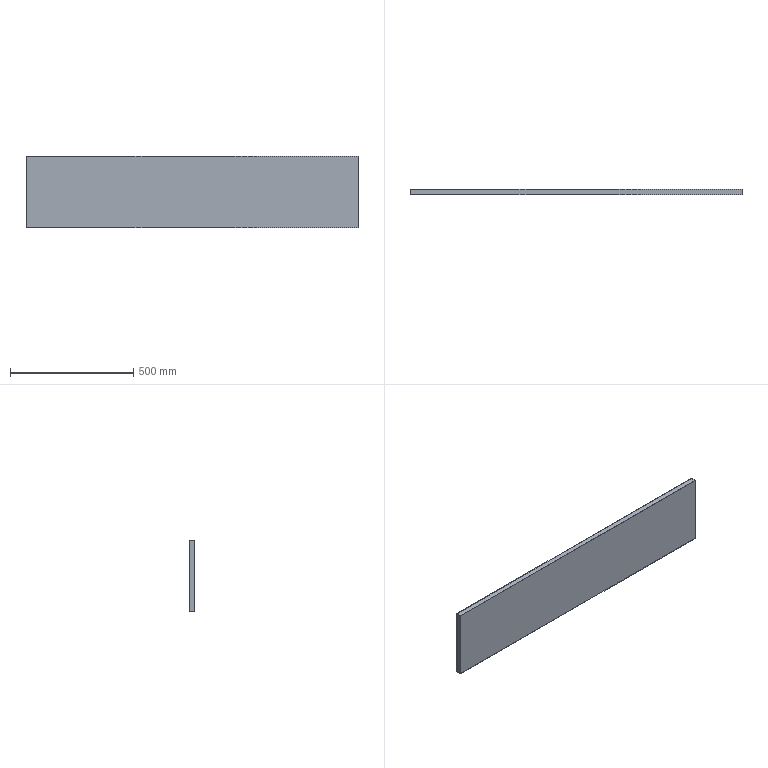Part | SolidWorks | features Extrusion 1, ICE 1, Shell 1 | 1 solid | 12 faces | box 1346 x 22 x 288 mm | volume 1667952 mm3 | plane 12
STEP:
#1=CARTESIAN_POINT('',(-673.,0.,-144.));
#2=VERTEX_POINT('',#1);
#3=CARTESIAN_POINT('',(-673.,0.,144.));
#4=VERTEX_POINT('',#3);
#5=CARTESIAN_POINT('',(-673.,0.,-144.));
#6=DIRECTION('',(0.,0.,1.));
#7=VECTOR('',#6,1000.);
#8=LINE('',#5,#7);
#9=EDGE_CURVE('',#2,#4,#8,.T.);
#10=ORIENTED_EDGE('',*,*,#9,.F.);
#11=CARTESIAN_POINT('',(-673.,-22.,-144.));
#12=VERTEX_POINT('',#11);
#13=CARTESIAN_POINT('',(-673.,-20.,-144.));
#14=DIRECTION('',(0.,1.,0.));
#15=VECTOR('',#14,1000.);
#16=LINE('',#13,#15);
#17=EDGE_CURVE('',#12,#2,#16,.T.);
#18=ORIENTED_EDGE('',*,*,#17,.F.);
#19=CARTESIAN_POINT('',(-673.,-22.,144.));
#20=VERTEX_POINT('',#19);
#21=CARTESIAN_POINT('',(-673.,-22.,144.));
#22=DIRECTION('',(0.,0.,-1.));
#23=VECTOR('',#22,1000.);
#24=LINE('',#21,#23);
#25=EDGE_CURVE('',#20,#12,#24,.T.);
#26=ORIENTED_EDGE('',*,*,#25,.F.);
#27=CARTESIAN_POINT('',(-673.,-20.,144.));
#28=DIRECTION('',(0.,1.,0.));
#29=VECTOR('',#28,1000.);
#30=LINE('',#27,#29);
#31=EDGE_CURVE('',#20,#4,#30,.T.);
#32=ORIENTED_EDGE('',*,*,#31,.T.);
#33=EDGE_LOOP('',(#10,#18,#26,#32));
#34=FACE_OUTER_BOUND('',#33,.T.);
#35=CARTESIAN_POINT('',(-673.,-20.,-144.));
#36=DIRECTION('',(-1.,0.,0.));
#37=DIRECTION('',(0.,0.,1.));
#38=AXIS2_PLACEMENT_3D('',#35,#36,#37);
#39=PLANE('',#38);
#40=ADVANCED_FACE('',(#34),#39,.T.);
#41=CARTESIAN_POINT('',(673.,0.,-144.));
#42=VERTEX_POINT('',#41);
#43=CARTESIAN_POINT('',(-673.,0.,-144.));
#44=DIRECTION('',(-1.,0.,0.));
#45=VECTOR('',#44,1000.);
#46=LINE('',#43,#45);
#47=EDGE_CURVE('',#42,#2,#46,.T.);
#48=ORIENTED_EDGE('',*,*,#47,.F.);
#49=CARTESIAN_POINT('',(673.,-22.,-144.));
#50=VERTEX_POINT('',#49);
#51=CARTESIAN_POINT('',(673.,-20.,-144.));
#52=DIRECTION('',(0.,1.,0.));
#53=VECTOR('',#52,1000.);
#54=LINE('',#51,#53);
#55=EDGE_CURVE('',#50,#42,#54,.T.);
#56=ORIENTED_EDGE('',*,*,#55,.F.);
#57=CARTESIAN_POINT('',(-673.,-22.,-144.));
#58=DIRECTION('',(1.,0.,0.));
#59=VECTOR('',#58,1000.);
#60=LINE('',#57,#59);
#61=EDGE_CURVE('',#12,#50,#60,.T.);
#62=ORIENTED_EDGE('',*,*,#61,.F.);
#63=ORIENTED_EDGE('',*,*,#17,.T.);
#64=EDGE_LOOP('',(#48,#56,#62,#63));
#65=FACE_OUTER_BOUND('',#64,.T.);
#66=CARTESIAN_POINT('',(-673.,-20.,-144.));
#67=DIRECTION('',(0.,0.,-1.));
#68=DIRECTION('',(-1.,0.,0.));
#69=AXIS2_PLACEMENT_3D('',#66,#67,#68);
#70=PLANE('',#69);
#71=ADVANCED_FACE('',(#65),#70,.T.);
#72=CARTESIAN_POINT('',(673.,0.,144.));
#73=VERTEX_POINT('',#72);
#74=CARTESIAN_POINT('',(673.,0.,-144.));
#75=DIRECTION('',(0.,0.,-1.));
#76=VECTOR('',#75,1000.);
#77=LINE('',#74,#76);
#78=EDGE_CURVE('',#73,#42,#77,.T.);
#79=ORIENTED_EDGE('',*,*,#78,.F.);
#80=CARTESIAN_POINT('',(673.,-22.,144.));
#81=VERTEX_POINT('',#80);
#82=CARTESIAN_POINT('',(673.,-20.,144.));
#83=DIRECTION('',(0.,1.,0.));
#84=VECTOR('',#83,1000.);
#85=LINE('',#82,#84);
#86=EDGE_CURVE('',#81,#73,#85,.T.);
#87=ORIENTED_EDGE('',*,*,#86,.F.);
#88=CARTESIAN_POINT('',(673.,-22.,144.));
#89=DIRECTION('',(0.,0.,1.));
#90=VECTOR('',#89,1000.);
#91=LINE('',#88,#90);
#92=EDGE_CURVE('',#50,#81,#91,.T.);
#93=ORIENTED_EDGE('',*,*,#92,.F.);
#94=ORIENTED_EDGE('',*,*,#55,.T.);
#95=EDGE_LOOP('',(#79,#87,#93,#94));
#96=FACE_OUTER_BOUND('',#95,.T.);
#97=CARTESIAN_POINT('',(673.,-20.,-144.));
#98=DIRECTION('',(1.,0.,0.));
#99=DIRECTION('',(0.,0.,-1.));
#100=AXIS2_PLACEMENT_3D('',#97,#98,#99);
#101=PLANE('',#100);
#102=ADVANCED_FACE('',(#96),#101,.T.);
#103=CARTESIAN_POINT('',(-673.,0.,144.));
#104=DIRECTION('',(1.,0.,0.));
#105=VECTOR('',#104,1000.);
#106=LINE('',#103,#105);
#107=EDGE_CURVE('',#4,#73,#106,.T.);
#108=ORIENTED_EDGE('',*,*,#107,.F.);
#109=ORIENTED_EDGE('',*,*,#31,.F.);
#110=CARTESIAN_POINT('',(-673.,-22.,144.));
#111=DIRECTION('',(-1.,0.,0.));
#112=VECTOR('',#111,1000.);
#113=LINE('',#110,#112);
#114=EDGE_CURVE('',#81,#20,#113,.T.);
#115=ORIENTED_EDGE('',*,*,#114,.F.);
#116=ORIENTED_EDGE('',*,*,#86,.T.);
#117=EDGE_LOOP('',(#108,#109,#115,#116));
#118=FACE_OUTER_BOUND('',#117,.T.);
#119=CARTESIAN_POINT('',(-673.,-20.,144.));
#120=DIRECTION('',(0.,0.,1.));
#121=DIRECTION('',(1.,0.,0.));
#122=AXIS2_PLACEMENT_3D('',#119,#120,#121);
#123=PLANE('',#122);
#124=ADVANCED_FACE('',(#118),#123,.T.);
#125=ORIENTED_EDGE('',*,*,#9,.T.);
#126=ORIENTED_EDGE('',*,*,#107,.T.);
#127=ORIENTED_EDGE('',*,*,#78,.T.);
#128=ORIENTED_EDGE('',*,*,#47,.T.);
#129=EDGE_LOOP('',(#125,#126,#127,#128));
#130=FACE_OUTER_BOUND('',#129,.T.);
#131=CARTESIAN_POINT('',(-673.,0.,144.));
#132=DIRECTION('',(0.,1.,0.));
#133=DIRECTION('',(0.,0.,1.));
#134=AXIS2_PLACEMENT_3D('',#131,#132,#133);
#135=PLANE('',#134);
#136=ADVANCED_FACE('',(#130),#135,.T.);
#137=ORIENTED_EDGE('',*,*,#25,.T.);
#138=ORIENTED_EDGE('',*,*,#61,.T.);
#139=ORIENTED_EDGE('',*,*,#92,.T.);
#140=ORIENTED_EDGE('',*,*,#114,.T.);
#141=EDGE_LOOP('',(#137,#138,#139,#140));
#142=FACE_OUTER_BOUND('',#141,.T.);
#143=CARTESIAN_POINT('',(-673.,-22.,-144.));
#144=DIRECTION('',(0.,-1.,0.));
#145=DIRECTION('',(0.,0.,-1.));
#146=AXIS2_PLACEMENT_3D('',#143,#144,#145);
#147=PLANE('',#146);
#148=ADVANCED_FACE('',(#142),#147,.T.);
#149=CLOSED_SHELL('',(#40,#71,#102,#124,#136,#148));
#150=CARTESIAN_POINT('',(671.,-20.,-142.));
#151=VERTEX_POINT('',#150);
#152=CARTESIAN_POINT('',(-671.,-20.,-142.));
#153=VERTEX_POINT('',#152);
#154=CARTESIAN_POINT('',(-673.,-20.,-142.));
#155=DIRECTION('',(-1.,0.,0.));
#156=VECTOR('',#155,1000.);
#157=LINE('',#154,#156);
#158=EDGE_CURVE('',#151,#153,#157,.T.);
#159=ORIENTED_EDGE('',*,*,#158,.T.);
#160=CARTESIAN_POINT('',(-671.,-20.,142.));
#161=VERTEX_POINT('',#160);
#162=CARTESIAN_POINT('',(-671.,-20.,144.));
#163=DIRECTION('',(0.,0.,1.));
#164=VECTOR('',#163,1000.);
#165=LINE('',#162,#164);
#166=EDGE_CURVE('',#153,#161,#165,.T.);
#167=ORIENTED_EDGE('',*,*,#166,.T.);
#168=CARTESIAN_POINT('',(671.,-20.,142.));
#169=VERTEX_POINT('',#168);
#170=CARTESIAN_POINT('',(-673.,-20.,142.));
#171=DIRECTION('',(1.,0.,0.));
#172=VECTOR('',#171,1000.);
#173=LINE('',#170,#172);
#174=EDGE_CURVE('',#161,#169,#173,.T.);
#175=ORIENTED_EDGE('',*,*,#174,.T.);
#176=CARTESIAN_POINT('',(671.,-20.,144.));
#177=DIRECTION('',(0.,0.,-1.));
#178=VECTOR('',#177,1000.);
#179=LINE('',#176,#178);
#180=EDGE_CURVE('',#169,#151,#179,.T.);
#181=ORIENTED_EDGE('',*,*,#180,.T.);
#182=EDGE_LOOP('',(#159,#167,#175,#181));
#183=FACE_OUTER_BOUND('',#182,.T.);
#184=CARTESIAN_POINT('',(-673.,-20.,-144.));
#185=DIRECTION('',(0.,-1.,0.));
#186=DIRECTION('',(0.,0.,-1.));
#187=AXIS2_PLACEMENT_3D('',#184,#185,#186);
#188=PLANE('',#187);
#189=ADVANCED_FACE('',(#183),#188,.F.);
#190=CARTESIAN_POINT('',(-671.,-2.,-142.));
#191=VERTEX_POINT('',#190);
#192=CARTESIAN_POINT('',(-671.,-2.,142.));
#193=VERTEX_POINT('',#192);
#194=CARTESIAN_POINT('',(-671.,-2.,144.));
#195=DIRECTION('',(0.,0.,1.));
#196=VECTOR('',#195,1000.);
#197=LINE('',#194,#196);
#198=EDGE_CURVE('',#191,#193,#197,.T.);
#199=ORIENTED_EDGE('',*,*,#198,.F.);
#200=CARTESIAN_POINT('',(671.,-2.,-142.));
#201=VERTEX_POINT('',#200);
#202=CARTESIAN_POINT('',(-673.,-2.,-142.));
#203=DIRECTION('',(-1.,0.,0.));
#204=VECTOR('',#203,1000.);
#205=LINE('',#202,#204);
#206=EDGE_CURVE('',#201,#191,#205,.T.);
#207=ORIENTED_EDGE('',*,*,#206,.F.);
#208=CARTESIAN_POINT('',(671.,-2.,142.));
#209=VERTEX_POINT('',#208);
#210=CARTESIAN_POINT('',(671.,-2.,144.));
#211=DIRECTION('',(0.,0.,-1.));
#212=VECTOR('',#211,1000.);
#213=LINE('',#210,#212);
#214=EDGE_CURVE('',#209,#201,#213,.T.);
#215=ORIENTED_EDGE('',*,*,#214,.F.);
#216=CARTESIAN_POINT('',(-673.,-2.,142.));
#217=DIRECTION('',(1.,0.,0.));
#218=VECTOR('',#217,1000.);
#219=LINE('',#216,#218);
#220=EDGE_CURVE('',#193,#209,#219,.T.);
#221=ORIENTED_EDGE('',*,*,#220,.F.);
#222=EDGE_LOOP('',(#199,#207,#215,#221));
#223=FACE_OUTER_BOUND('',#222,.T.);
#224=CARTESIAN_POINT('',(-673.,-2.,144.));
#225=DIRECTION('',(0.,1.,0.));
#226=DIRECTION('',(0.,0.,1.));
#227=AXIS2_PLACEMENT_3D('',#224,#225,#226);
#228=PLANE('',#227);
#229=ADVANCED_FACE('',(#223),#228,.F.);
#230=ORIENTED_EDGE('',*,*,#220,.T.);
#231=CARTESIAN_POINT('',(671.,-20.,142.));
#232=DIRECTION('',(0.,1.,0.));
#233=VECTOR('',#232,1000.);
#234=LINE('',#231,#233);
#235=EDGE_CURVE('',#169,#209,#234,.T.);
#236=ORIENTED_EDGE('',*,*,#235,.F.);
#237=ORIENTED_EDGE('',*,*,#174,.F.);
#238=CARTESIAN_POINT('',(-671.,-20.,142.));
#239=DIRECTION('',(0.,1.,0.));
#240=VECTOR('',#239,1000.);
#241=LINE('',#238,#240);
#242=EDGE_CURVE('',#161,#193,#241,.T.);
#243=ORIENTED_EDGE('',*,*,#242,.T.);
#244=EDGE_LOOP('',(#230,#236,#237,#243));
#245=FACE_OUTER_BOUND('',#244,.T.);
#246=CARTESIAN_POINT('',(-673.,-20.,142.));
#247=DIRECTION('',(0.,0.,1.));
#248=DIRECTION('',(1.,0.,0.));
#249=AXIS2_PLACEMENT_3D('',#246,#247,#248);
#250=PLANE('',#249);
#251=ADVANCED_FACE('',(#245),#250,.F.);
#252=ORIENTED_EDGE('',*,*,#214,.T.);
#253=CARTESIAN_POINT('',(671.,-20.,-142.));
#254=DIRECTION('',(0.,1.,0.));
#255=VECTOR('',#254,1000.);
#256=LINE('',#253,#255);
#257=EDGE_CURVE('',#151,#201,#256,.T.);
#258=ORIENTED_EDGE('',*,*,#257,.F.);
#259=ORIENTED_EDGE('',*,*,#180,.F.);
#260=ORIENTED_EDGE('',*,*,#235,.T.);
#261=EDGE_LOOP('',(#252,#258,#259,#260));
#262=FACE_OUTER_BOUND('',#261,.T.);
#263=CARTESIAN_POINT('',(671.,-20.,-144.));
#264=DIRECTION('',(1.,0.,0.));
#265=DIRECTION('',(0.,0.,-1.));
#266=AXIS2_PLACEMENT_3D('',#263,#264,#265);
#267=PLANE('',#266);
#268=ADVANCED_FACE('',(#262),#267,.F.);
#269=ORIENTED_EDGE('',*,*,#206,.T.);
#270=CARTESIAN_POINT('',(-671.,-20.,-142.));
#271=DIRECTION('',(0.,1.,0.));
#272=VECTOR('',#271,1000.);
#273=LINE('',#270,#272);
#274=EDGE_CURVE('',#153,#191,#273,.T.);
#275=ORIENTED_EDGE('',*,*,#274,.F.);
#276=ORIENTED_EDGE('',*,*,#158,.F.);
#277=ORIENTED_EDGE('',*,*,#257,.T.);
#278=EDGE_LOOP('',(#269,#275,#276,#277));
#279=FACE_OUTER_BOUND('',#278,.T.);
#280=CARTESIAN_POINT('',(-673.,-20.,-142.));
#281=DIRECTION('',(0.,0.,-1.));
#282=DIRECTION('',(-1.,0.,0.));
#283=AXIS2_PLACEMENT_3D('',#280,#281,#282);
#284=PLANE('',#283);
#285=ADVANCED_FACE('',(#279),#284,.F.);
#286=ORIENTED_EDGE('',*,*,#198,.T.);
#287=ORIENTED_EDGE('',*,*,#242,.F.);
#288=ORIENTED_EDGE('',*,*,#166,.F.);
#289=ORIENTED_EDGE('',*,*,#274,.T.);
#290=EDGE_LOOP('',(#286,#287,#288,#289));
#291=FACE_OUTER_BOUND('',#290,.T.);
#292=CARTESIAN_POINT('',(-671.,-20.,-144.));
#293=DIRECTION('',(-1.,0.,0.));
#294=DIRECTION('',(0.,0.,1.));
#295=AXIS2_PLACEMENT_3D('',#292,#293,#294);
#296=PLANE('',#295);
#297=ADVANCED_FACE('',(#291),#296,.F.);
#298=CLOSED_SHELL('',(#189,#229,#251,#268,#285,#297));
#299=ORIENTED_CLOSED_SHELL('',*,#298,.F.);
#300=BREP_WITH_VOIDS('',#149,(#299));
#301=CARTESIAN_POINT('',(0.,0.,0.));
#302=DIRECTION('',(0.,0.,1.));
#303=DIRECTION('',(1.,0.,0.));
#304=AXIS2_PLACEMENT_3D('',#301,#302,#303);
#305=(LENGTH_UNIT()NAMED_UNIT(*)SI_UNIT(.MILLI.,.METRE.));
#306=UNCERTAINTY_MEASURE_WITH_UNIT(LENGTH_MEASURE(0.00001),#305,'','');
#307=(NAMED_UNIT(*)PLANE_ANGLE_UNIT()SI_UNIT($,.RADIAN.));
#308=(NAMED_UNIT(*)SI_UNIT($,.STERADIAN.)SOLID_ANGLE_UNIT());
#309=(GEOMETRIC_REPRESENTATION_CONTEXT(3)GLOBAL_UNCERTAINTY_ASSIGNED_CONTEXT((#306))GLOBAL_UNIT_ASSIGNED_CONTEXT((#305,#307,#308))REPRESENTATION_CONTEXT('',''));
#310=ADVANCED_BREP_SHAPE_REPRESENTATION('',(#300,#304),#309);